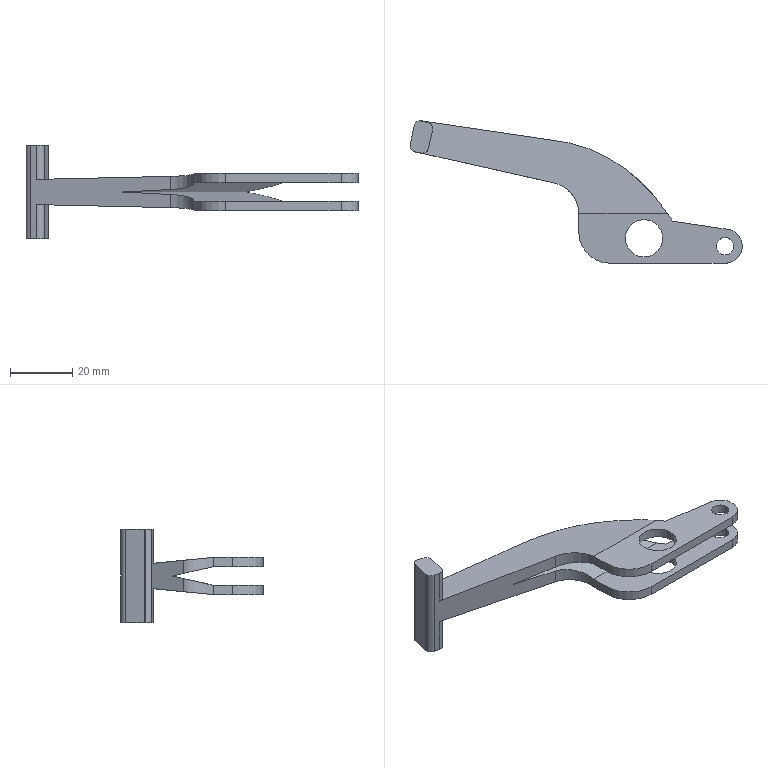Part | SolidWorks | features Fillet 3, ICE 3, Extrusion 1 | 1 solid | 45 faces | box 106.747 x 45.786 x 30 mm | volume 13050 mm3 | plane 23 | cylinder 21 | spline 1 | commonest cylinder face diameters 4 x7 5.55 x4 12 x4 20 x4 11 x2